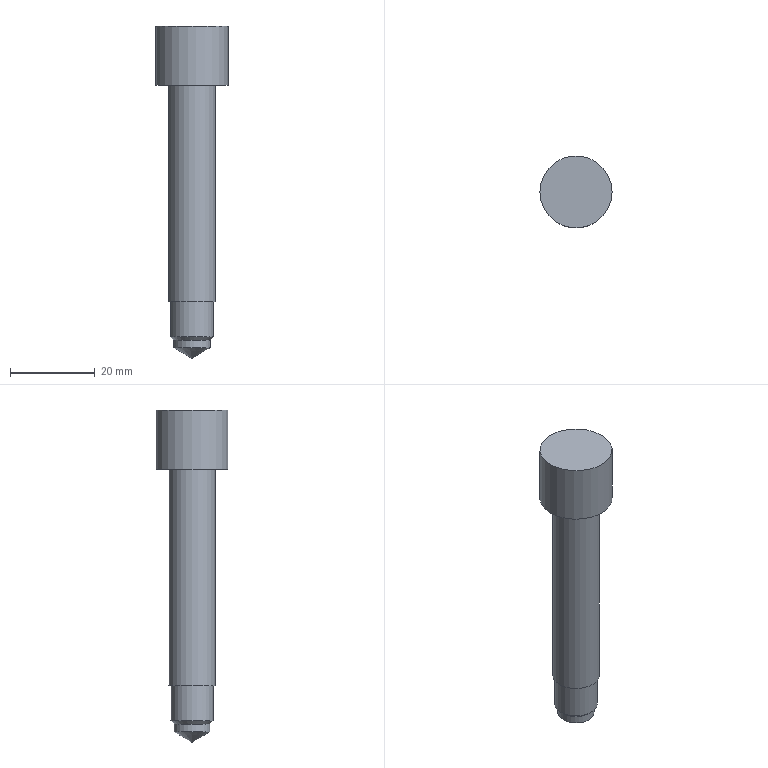Part | NX | features BREP 2 | 2 solids | 21 faces | box 17 x 17 x 78.231 mm | volume 15034 mm3 | plane 14 | cylinder 5 | cone 2 | commonest cylinder face diameters 8.5 x1 10 x1 11 x1 16 x1 17 x1
STEP:
#1=CARTESIAN_POINT('',(-4.25,0.,0.));
#2=VERTEX_POINT('',#1);
#3=CARTESIAN_POINT('',(0.,0.,0.));
#4=DIRECTION('',(0.,0.,1.));
#5=DIRECTION('',(-1.,0.,0.));
#6=AXIS2_PLACEMENT_3D('',#3,#4,#5);
#7=CIRCLE('',#6,4.25);
#8=EDGE_CURVE('',#2,#2,#7,.T.);
#9=ORIENTED_EDGE('',*,*,#8,.F.);
#10=EDGE_LOOP('',(#9));
#11=FACE_BOUND('',#10,.T.);
#12=CARTESIAN_POINT('',(-4.25,0.,-10.8));
#13=VERTEX_POINT('',#12);
#14=CARTESIAN_POINT('',(0.,0.,-10.8));
#15=DIRECTION('',(0.,0.,-1.));
#16=DIRECTION('',(-1.,0.,0.));
#17=AXIS2_PLACEMENT_3D('',#14,#15,#16);
#18=CIRCLE('',#17,4.25);
#19=EDGE_CURVE('',#13,#13,#18,.T.);
#20=ORIENTED_EDGE('',*,*,#19,.F.);
#21=EDGE_LOOP('',(#20));
#22=FACE_BOUND('',#21,.T.);
#23=CARTESIAN_POINT('',(0.,0.,-10.8));
#24=DIRECTION('',(0.,0.,1.));
#25=DIRECTION('',(-1.,0.,0.));
#26=AXIS2_PLACEMENT_3D('',#23,#24,#25);
#27=CYLINDRICAL_SURFACE('',#26,4.25);
#28=ADVANCED_FACE('',(#11,#22),#27,.T.);
#29=CARTESIAN_POINT('',(-0.2034,0.,-13.231));
#30=VERTEX_POINT('',#29);
#31=CARTESIAN_POINT('',(0.,0.,-13.231));
#32=DIRECTION('',(0.,0.,-1.));
#33=DIRECTION('',(-1.,0.,0.));
#34=AXIS2_PLACEMENT_3D('',#31,#32,#33);
#35=CIRCLE('',#34,0.2034);
#36=EDGE_CURVE('',#30,#30,#35,.T.);
#37=ORIENTED_EDGE('',*,*,#36,.T.);
#38=EDGE_LOOP('',(#37));
#39=FACE_BOUND('',#38,.T.);
#40=CARTESIAN_POINT('',(0.,0.,-13.231));
#41=DIRECTION('',(0.,0.,-1.));
#42=DIRECTION('',(1.,0.,0.));
#43=AXIS2_PLACEMENT_3D('',#40,#41,#42);
#44=PLANE('',#43);
#45=ADVANCED_FACE('',(#39),#44,.T.);
#46=ORIENTED_EDGE('',*,*,#36,.F.);
#47=EDGE_LOOP('',(#46));
#48=FACE_BOUND('',#47,.T.);
#49=ORIENTED_EDGE('',*,*,#19,.T.);
#50=EDGE_LOOP('',(#49));
#51=FACE_BOUND('',#50,.T.);
#52=CARTESIAN_POINT('',(0.,0.,-10.8));
#53=DIRECTION('',(0.,0.,1.));
#54=DIRECTION('',(-1.,0.,0.));
#55=AXIS2_PLACEMENT_3D('',#52,#53,#54);
#56=CONICAL_SURFACE('',#55,4.25,1.03);
#57=ADVANCED_FACE('',(#48,#51),#56,.T.);
#58=ORIENTED_EDGE('',*,*,#8,.T.);
#59=EDGE_LOOP('',(#58));
#60=FACE_BOUND('',#59,.T.);
#61=CARTESIAN_POINT('',(-5.5,0.,0.));
#62=VERTEX_POINT('',#61);
#63=CARTESIAN_POINT('',(0.,0.,0.));
#64=DIRECTION('',(0.,0.,-1.));
#65=DIRECTION('',(-1.,0.,0.));
#66=AXIS2_PLACEMENT_3D('',#63,#64,#65);
#67=CIRCLE('',#66,5.5);
#68=EDGE_CURVE('',#62,#62,#67,.T.);
#69=ORIENTED_EDGE('',*,*,#68,.T.);
#70=EDGE_LOOP('',(#69));
#71=FACE_BOUND('',#70,.T.);
#72=CARTESIAN_POINT('',(0.,0.,0.));
#73=DIRECTION('',(0.,0.,-1.));
#74=DIRECTION('',(1.,0.,0.));
#75=AXIS2_PLACEMENT_3D('',#72,#73,#74);
#76=PLANE('',#75);
#77=ADVANCED_FACE('',(#60,#71),#76,.T.);
#78=ORIENTED_EDGE('',*,*,#68,.F.);
#79=EDGE_LOOP('',(#78));
#80=FACE_BOUND('',#79,.T.);
#81=CARTESIAN_POINT('',(-5.5,0.,51.));
#82=VERTEX_POINT('',#81);
#83=CARTESIAN_POINT('',(0.,0.,51.));
#84=DIRECTION('',(0.,0.,-1.));
#85=DIRECTION('',(-1.,0.,0.));
#86=AXIS2_PLACEMENT_3D('',#83,#84,#85);
#87=CIRCLE('',#86,5.5);
#88=EDGE_CURVE('',#82,#82,#87,.T.);
#89=ORIENTED_EDGE('',*,*,#88,.T.);
#90=EDGE_LOOP('',(#89));
#91=FACE_BOUND('',#90,.T.);
#92=CARTESIAN_POINT('',(0.,0.,51.));
#93=DIRECTION('',(0.,0.,-1.));
#94=DIRECTION('',(1.,0.,0.));
#95=AXIS2_PLACEMENT_3D('',#92,#93,#94);
#96=CYLINDRICAL_SURFACE('',#95,5.5);
#97=ADVANCED_FACE('',(#80,#91),#96,.T.);
#98=CARTESIAN_POINT('',(8.5,0.,65.));
#99=VERTEX_POINT('',#98);
#100=CARTESIAN_POINT('',(0.,0.,65.));
#101=DIRECTION('',(0.,0.,1.));
#102=DIRECTION('',(1.,0.,0.));
#103=AXIS2_PLACEMENT_3D('',#100,#101,#102);
#104=CIRCLE('',#103,8.5);
#105=EDGE_CURVE('',#99,#99,#104,.T.);
#106=ORIENTED_EDGE('',*,*,#105,.T.);
#107=EDGE_LOOP('',(#106));
#108=FACE_BOUND('',#107,.T.);
#109=CARTESIAN_POINT('',(0.,0.,65.));
#110=DIRECTION('',(0.,0.,1.));
#111=DIRECTION('',(-1.,0.,0.));
#112=AXIS2_PLACEMENT_3D('',#109,#110,#111);
#113=PLANE('',#112);
#114=ADVANCED_FACE('',(#108),#113,.T.);
#115=ORIENTED_EDGE('',*,*,#105,.F.);
#116=EDGE_LOOP('',(#115));
#117=FACE_BOUND('',#116,.T.);
#118=CARTESIAN_POINT('',(8.5,0.,51.));
#119=VERTEX_POINT('',#118);
#120=CARTESIAN_POINT('',(0.,0.,51.));
#121=DIRECTION('',(0.,0.,1.));
#122=DIRECTION('',(1.,0.,0.));
#123=AXIS2_PLACEMENT_3D('',#120,#121,#122);
#124=CIRCLE('',#123,8.5);
#125=EDGE_CURVE('',#119,#119,#124,.T.);
#126=ORIENTED_EDGE('',*,*,#125,.T.);
#127=EDGE_LOOP('',(#126));
#128=FACE_BOUND('',#127,.T.);
#129=CARTESIAN_POINT('',(0.,0.,51.));
#130=DIRECTION('',(0.,0.,1.));
#131=DIRECTION('',(-1.,0.,0.));
#132=AXIS2_PLACEMENT_3D('',#129,#130,#131);
#133=CYLINDRICAL_SURFACE('',#132,8.5);
#134=ADVANCED_FACE('',(#117,#128),#133,.T.);
#135=ORIENTED_EDGE('',*,*,#88,.F.);
#136=EDGE_LOOP('',(#135));
#137=FACE_BOUND('',#136,.T.);
#138=ORIENTED_EDGE('',*,*,#125,.F.);
#139=EDGE_LOOP('',(#138));
#140=FACE_BOUND('',#139,.T.);
#141=CARTESIAN_POINT('',(0.,0.,51.));
#142=DIRECTION('',(0.,0.,-1.));
#143=DIRECTION('',(1.,0.,0.));
#144=AXIS2_PLACEMENT_3D('',#141,#142,#143);
#145=PLANE('',#144);
#146=ADVANCED_FACE('',(#137,#140),#145,.T.);
#147=CLOSED_SHELL('',(#28,#45,#57,#77,#97,#114,#134,#146));
#148=MANIFOLD_SOLID_BREP('',#147);
#149=CARTESIAN_POINT('',(8.,0.,61.));
#150=VERTEX_POINT('',#149);
#151=CARTESIAN_POINT('',(0.,0.,61.));
#152=DIRECTION('',(0.,0.,1.));
#153=DIRECTION('',(1.,0.,0.));
#154=AXIS2_PLACEMENT_3D('',#151,#152,#153);
#155=CIRCLE('',#154,8.);
#156=EDGE_CURVE('',#150,#150,#155,.T.);
#157=ORIENTED_EDGE('',*,*,#156,.T.);
#158=EDGE_LOOP('',(#157));
#159=FACE_BOUND('',#158,.T.);
#160=CARTESIAN_POINT('',(4.619,0.,61.));
#161=VERTEX_POINT('',#160);
#162=CARTESIAN_POINT('',(2.309,-4.,61.));
#163=VERTEX_POINT('',#162);
#164=CARTESIAN_POINT('',(4.619,0.,61.));
#165=DIRECTION('',(-0.5,-0.866,0.));
#166=VECTOR('',#165,1000.);
#167=LINE('',#164,#166);
#168=EDGE_CURVE('',#161,#163,#167,.T.);
#169=ORIENTED_EDGE('',*,*,#168,.T.);
#170=CARTESIAN_POINT('',(-2.309,-4.,61.));
#171=VERTEX_POINT('',#170);
#172=CARTESIAN_POINT('',(2.309,-4.,61.));
#173=DIRECTION('',(-1.,0.,0.));
#174=VECTOR('',#173,1000.);
#175=LINE('',#172,#174);
#176=EDGE_CURVE('',#163,#171,#175,.T.);
#177=ORIENTED_EDGE('',*,*,#176,.T.);
#178=CARTESIAN_POINT('',(-4.619,0.,61.));
#179=VERTEX_POINT('',#178);
#180=CARTESIAN_POINT('',(-2.309,-4.,61.));
#181=DIRECTION('',(-0.5,0.866,0.));
#182=VECTOR('',#181,1000.);
#183=LINE('',#180,#182);
#184=EDGE_CURVE('',#171,#179,#183,.T.);
#185=ORIENTED_EDGE('',*,*,#184,.T.);
#186=CARTESIAN_POINT('',(-2.309,4.,61.));
#187=VERTEX_POINT('',#186);
#188=CARTESIAN_POINT('',(-4.619,0.,61.));
#189=DIRECTION('',(0.5,0.866,0.));
#190=VECTOR('',#189,1000.);
#191=LINE('',#188,#190);
#192=EDGE_CURVE('',#179,#187,#191,.T.);
#193=ORIENTED_EDGE('',*,*,#192,.T.);
#194=CARTESIAN_POINT('',(2.309,4.,61.));
#195=VERTEX_POINT('',#194);
#196=CARTESIAN_POINT('',(-2.309,4.,61.));
#197=DIRECTION('',(1.,0.,0.));
#198=VECTOR('',#197,1000.);
#199=LINE('',#196,#198);
#200=EDGE_CURVE('',#187,#195,#199,.T.);
#201=ORIENTED_EDGE('',*,*,#200,.T.);
#202=CARTESIAN_POINT('',(2.309,4.,61.));
#203=DIRECTION('',(0.5,-0.866,0.));
#204=VECTOR('',#203,1000.);
#205=LINE('',#202,#204);
#206=EDGE_CURVE('',#195,#161,#205,.T.);
#207=ORIENTED_EDGE('',*,*,#206,.T.);
#208=EDGE_LOOP('',(#169,#177,#185,#193,#201,#207));
#209=FACE_BOUND('',#208,.T.);
#210=CARTESIAN_POINT('',(0.,0.,61.));
#211=DIRECTION('',(0.,0.,1.));
#212=DIRECTION('',(-1.,0.,0.));
#213=AXIS2_PLACEMENT_3D('',#210,#211,#212);
#214=PLANE('',#213);
#215=ADVANCED_FACE('',(#159,#209),#214,.T.);
#216=CARTESIAN_POINT('',(5.,0.,-8.25));
#217=VERTEX_POINT('',#216);
#218=CARTESIAN_POINT('',(0.,0.,-8.25));
#219=DIRECTION('',(0.,0.,1.));
#220=DIRECTION('',(1.,0.,0.));
#221=AXIS2_PLACEMENT_3D('',#218,#219,#220);
#222=CIRCLE('',#221,5.);
#223=EDGE_CURVE('',#217,#217,#222,.T.);
#224=ORIENTED_EDGE('',*,*,#223,.T.);
#225=EDGE_LOOP('',(#224));
#226=FACE_BOUND('',#225,.T.);
#227=CARTESIAN_POINT('',(5.,0.,51.));
#228=VERTEX_POINT('',#227);
#229=CARTESIAN_POINT('',(0.,0.,51.));
#230=DIRECTION('',(0.,0.,1.));
#231=DIRECTION('',(1.,0.,0.));
#232=AXIS2_PLACEMENT_3D('',#229,#230,#231);
#233=CIRCLE('',#232,5.);
#234=EDGE_CURVE('',#228,#228,#233,.T.);
#235=ORIENTED_EDGE('',*,*,#234,.F.);
#236=EDGE_LOOP('',(#235));
#237=FACE_BOUND('',#236,.T.);
#238=CARTESIAN_POINT('',(0.,0.,-9.));
#239=DIRECTION('',(0.,0.,1.));
#240=DIRECTION('',(-1.,0.,0.));
#241=AXIS2_PLACEMENT_3D('',#238,#239,#240);
#242=CYLINDRICAL_SURFACE('',#241,5.);
#243=ADVANCED_FACE('',(#226,#237),#242,.T.);
#244=CARTESIAN_POINT('',(4.25,0.,-9.));
#245=VERTEX_POINT('',#244);
#246=CARTESIAN_POINT('',(0.,0.,-9.));
#247=DIRECTION('',(0.,0.,-1.));
#248=DIRECTION('',(1.,0.,0.));
#249=AXIS2_PLACEMENT_3D('',#246,#247,#248);
#250=CIRCLE('',#249,4.25);
#251=EDGE_CURVE('',#245,#245,#250,.T.);
#252=ORIENTED_EDGE('',*,*,#251,.T.);
#253=EDGE_LOOP('',(#252));
#254=FACE_BOUND('',#253,.T.);
#255=CARTESIAN_POINT('',(0.,0.,-9.));
#256=DIRECTION('',(0.,0.,1.));
#257=DIRECTION('',(-1.,0.,0.));
#258=AXIS2_PLACEMENT_3D('',#255,#256,#257);
#259=PLANE('',#258);
#260=ADVANCED_FACE('',(#254),#259,.F.);
#261=ORIENTED_EDGE('',*,*,#234,.T.);
#262=EDGE_LOOP('',(#261));
#263=FACE_BOUND('',#262,.T.);
#264=CARTESIAN_POINT('',(8.,0.,51.));
#265=VERTEX_POINT('',#264);
#266=CARTESIAN_POINT('',(0.,0.,51.));
#267=DIRECTION('',(0.,0.,1.));
#268=DIRECTION('',(1.,0.,0.));
#269=AXIS2_PLACEMENT_3D('',#266,#267,#268);
#270=CIRCLE('',#269,8.);
#271=EDGE_CURVE('',#265,#265,#270,.T.);
#272=ORIENTED_EDGE('',*,*,#271,.F.);
#273=EDGE_LOOP('',(#272));
#274=FACE_BOUND('',#273,.T.);
#275=CARTESIAN_POINT('',(0.,0.,51.));
#276=DIRECTION('',(0.,0.,-1.));
#277=DIRECTION('',(1.,0.,0.));
#278=AXIS2_PLACEMENT_3D('',#275,#276,#277);
#279=PLANE('',#278);
#280=ADVANCED_FACE('',(#263,#274),#279,.T.);
#281=ORIENTED_EDGE('',*,*,#156,.F.);
#282=EDGE_LOOP('',(#281));
#283=FACE_BOUND('',#282,.T.);
#284=ORIENTED_EDGE('',*,*,#271,.T.);
#285=EDGE_LOOP('',(#284));
#286=FACE_BOUND('',#285,.T.);
#287=CARTESIAN_POINT('',(0.,0.,51.));
#288=DIRECTION('',(0.,0.,1.));
#289=DIRECTION('',(-1.,0.,0.));
#290=AXIS2_PLACEMENT_3D('',#287,#288,#289);
#291=CYLINDRICAL_SURFACE('',#290,8.);
#292=ADVANCED_FACE('',(#283,#286),#291,.T.);
#293=ORIENTED_EDGE('',*,*,#251,.F.);
#294=EDGE_LOOP('',(#293));
#295=FACE_BOUND('',#294,.T.);
#296=ORIENTED_EDGE('',*,*,#223,.F.);
#297=EDGE_LOOP('',(#296));
#298=FACE_BOUND('',#297,.T.);
#299=CARTESIAN_POINT('',(0.,0.,-8.25));
#300=DIRECTION('',(0.,0.,1.));
#301=DIRECTION('',(-1.,0.,0.));
#302=AXIS2_PLACEMENT_3D('',#299,#300,#301);
#303=CONICAL_SURFACE('',#302,5.,0.7854);
#304=ADVANCED_FACE('',(#295,#298),#303,.T.);
#305=ORIENTED_EDGE('',*,*,#176,.F.);
#306=CARTESIAN_POINT('',(2.309,-4.,54.4));
#307=VERTEX_POINT('',#306);
#308=CARTESIAN_POINT('',(2.309,-4.,54.4));
#309=DIRECTION('',(0.,0.,1.));
#310=VECTOR('',#309,1000.);
#311=LINE('',#308,#310);
#312=EDGE_CURVE('',#307,#163,#311,.T.);
#313=ORIENTED_EDGE('',*,*,#312,.F.);
#314=CARTESIAN_POINT('',(-2.309,-4.,54.4));
#315=VERTEX_POINT('',#314);
#316=CARTESIAN_POINT('',(2.309,-4.,54.4));
#317=DIRECTION('',(-1.,0.,0.));
#318=VECTOR('',#317,1000.);
#319=LINE('',#316,#318);
#320=EDGE_CURVE('',#307,#315,#319,.T.);
#321=ORIENTED_EDGE('',*,*,#320,.T.);
#322=CARTESIAN_POINT('',(-2.309,-4.,54.4));
#323=DIRECTION('',(0.,0.,1.));
#324=VECTOR('',#323,1000.);
#325=LINE('',#322,#324);
#326=EDGE_CURVE('',#315,#171,#325,.T.);
#327=ORIENTED_EDGE('',*,*,#326,.T.);
#328=EDGE_LOOP('',(#305,#313,#321,#327));
#329=FACE_BOUND('',#328,.T.);
#330=CARTESIAN_POINT('',(2.309,-4.,54.4));
#331=DIRECTION('',(0.,1.,0.));
#332=DIRECTION('',(0.,0.,-1.));
#333=AXIS2_PLACEMENT_3D('',#330,#331,#332);
#334=PLANE('',#333);
#335=ADVANCED_FACE('',(#329),#334,.T.);
#336=ORIENTED_EDGE('',*,*,#184,.F.);
#337=ORIENTED_EDGE('',*,*,#326,.F.);
#338=CARTESIAN_POINT('',(-4.619,0.,54.4));
#339=VERTEX_POINT('',#338);
#340=CARTESIAN_POINT('',(-2.309,-4.,54.4));
#341=DIRECTION('',(-0.5,0.866,0.));
#342=VECTOR('',#341,1000.);
#343=LINE('',#340,#342);
#344=EDGE_CURVE('',#315,#339,#343,.T.);
#345=ORIENTED_EDGE('',*,*,#344,.T.);
#346=CARTESIAN_POINT('',(-4.619,0.,54.4));
#347=DIRECTION('',(0.,0.,1.));
#348=VECTOR('',#347,1000.);
#349=LINE('',#346,#348);
#350=EDGE_CURVE('',#339,#179,#349,.T.);
#351=ORIENTED_EDGE('',*,*,#350,.T.);
#352=EDGE_LOOP('',(#336,#337,#345,#351));
#353=FACE_BOUND('',#352,.T.);
#354=CARTESIAN_POINT('',(-2.309,-4.,54.4));
#355=DIRECTION('',(0.866,0.5,0.));
#356=DIRECTION('',(0.5,-0.866,0.));
#357=AXIS2_PLACEMENT_3D('',#354,#355,#356);
#358=PLANE('',#357);
#359=ADVANCED_FACE('',(#353),#358,.T.);
#360=ORIENTED_EDGE('',*,*,#192,.F.);
#361=ORIENTED_EDGE('',*,*,#350,.F.);
#362=CARTESIAN_POINT('',(-2.309,4.,54.4));
#363=VERTEX_POINT('',#362);
#364=CARTESIAN_POINT('',(-4.619,0.,54.4));
#365=DIRECTION('',(0.5,0.866,0.));
#366=VECTOR('',#365,1000.);
#367=LINE('',#364,#366);
#368=EDGE_CURVE('',#339,#363,#367,.T.);
#369=ORIENTED_EDGE('',*,*,#368,.T.);
#370=CARTESIAN_POINT('',(-2.309,4.,54.4));
#371=DIRECTION('',(0.,0.,1.));
#372=VECTOR('',#371,1000.);
#373=LINE('',#370,#372);
#374=EDGE_CURVE('',#363,#187,#373,.T.);
#375=ORIENTED_EDGE('',*,*,#374,.T.);
#376=EDGE_LOOP('',(#360,#361,#369,#375));
#377=FACE_BOUND('',#376,.T.);
#378=CARTESIAN_POINT('',(-4.619,0.,54.4));
#379=DIRECTION('',(0.866,-0.5,0.));
#380=DIRECTION('',(-0.5,-0.866,0.));
#381=AXIS2_PLACEMENT_3D('',#378,#379,#380);
#382=PLANE('',#381);
#383=ADVANCED_FACE('',(#377),#382,.T.);
#384=ORIENTED_EDGE('',*,*,#200,.F.);
#385=ORIENTED_EDGE('',*,*,#374,.F.);
#386=CARTESIAN_POINT('',(2.309,4.,54.4));
#387=VERTEX_POINT('',#386);
#388=CARTESIAN_POINT('',(-2.309,4.,54.4));
#389=DIRECTION('',(1.,0.,0.));
#390=VECTOR('',#389,1000.);
#391=LINE('',#388,#390);
#392=EDGE_CURVE('',#363,#387,#391,.T.);
#393=ORIENTED_EDGE('',*,*,#392,.T.);
#394=CARTESIAN_POINT('',(2.309,4.,54.4));
#395=DIRECTION('',(0.,0.,1.));
#396=VECTOR('',#395,1000.);
#397=LINE('',#394,#396);
#398=EDGE_CURVE('',#387,#195,#397,.T.);
#399=ORIENTED_EDGE('',*,*,#398,.T.);
#400=EDGE_LOOP('',(#384,#385,#393,#399));
#401=FACE_BOUND('',#400,.T.);
#402=CARTESIAN_POINT('',(-2.309,4.,54.4));
#403=DIRECTION('',(0.,-1.,0.));
#404=DIRECTION('',(0.,0.,1.));
#405=AXIS2_PLACEMENT_3D('',#402,#403,#404);
#406=PLANE('',#405);
#407=ADVANCED_FACE('',(#401),#406,.T.);
#408=ORIENTED_EDGE('',*,*,#206,.F.);
#409=ORIENTED_EDGE('',*,*,#398,.F.);
#410=CARTESIAN_POINT('',(4.619,0.,54.4));
#411=VERTEX_POINT('',#410);
#412=CARTESIAN_POINT('',(2.309,4.,54.4));
#413=DIRECTION('',(0.5,-0.866,0.));
#414=VECTOR('',#413,1000.);
#415=LINE('',#412,#414);
#416=EDGE_CURVE('',#387,#411,#415,.T.);
#417=ORIENTED_EDGE('',*,*,#416,.T.);
#418=CARTESIAN_POINT('',(4.619,0.,54.4));
#419=DIRECTION('',(0.,0.,1.));
#420=VECTOR('',#419,1000.);
#421=LINE('',#418,#420);
#422=EDGE_CURVE('',#411,#161,#421,.T.);
#423=ORIENTED_EDGE('',*,*,#422,.T.);
#424=EDGE_LOOP('',(#408,#409,#417,#423));
#425=FACE_BOUND('',#424,.T.);
#426=CARTESIAN_POINT('',(2.309,4.,54.4));
#427=DIRECTION('',(-0.866,-0.5,0.));
#428=DIRECTION('',(-0.5,0.866,0.));
#429=AXIS2_PLACEMENT_3D('',#426,#427,#428);
#430=PLANE('',#429);
#431=ADVANCED_FACE('',(#425),#430,.T.);
#432=ORIENTED_EDGE('',*,*,#168,.F.);
#433=ORIENTED_EDGE('',*,*,#422,.F.);
#434=CARTESIAN_POINT('',(4.619,0.,54.4));
#435=DIRECTION('',(-0.5,-0.866,0.));
#436=VECTOR('',#435,1000.);
#437=LINE('',#434,#436);
#438=EDGE_CURVE('',#411,#307,#437,.T.);
#439=ORIENTED_EDGE('',*,*,#438,.T.);
#440=ORIENTED_EDGE('',*,*,#312,.T.);
#441=EDGE_LOOP('',(#432,#433,#439,#440));
#442=FACE_BOUND('',#441,.T.);
#443=CARTESIAN_POINT('',(4.619,0.,54.4));
#444=DIRECTION('',(-0.866,0.5,0.));
#445=DIRECTION('',(0.5,0.866,0.));
#446=AXIS2_PLACEMENT_3D('',#443,#444,#445);
#447=PLANE('',#446);
#448=ADVANCED_FACE('',(#442),#447,.T.);
#449=ORIENTED_EDGE('',*,*,#320,.F.);
#450=ORIENTED_EDGE('',*,*,#438,.F.);
#451=ORIENTED_EDGE('',*,*,#416,.F.);
#452=ORIENTED_EDGE('',*,*,#392,.F.);
#453=ORIENTED_EDGE('',*,*,#368,.F.);
#454=ORIENTED_EDGE('',*,*,#344,.F.);
#455=EDGE_LOOP('',(#449,#450,#451,#452,#453,#454));
#456=FACE_BOUND('',#455,.T.);
#457=CARTESIAN_POINT('',(-6.928,-4.,54.4));
#458=DIRECTION('',(0.,0.,-1.));
#459=DIRECTION('',(1.,0.,0.));
#460=AXIS2_PLACEMENT_3D('',#457,#458,#459);
#461=PLANE('',#460);
#462=ADVANCED_FACE('',(#456),#461,.F.);
#463=CLOSED_SHELL('',(#215,#243,#260,#280,#292,#304,#335,#359,#383,#407,#431,#448,#462));
#464=MANIFOLD_SOLID_BREP('',#463);
#465=(LENGTH_UNIT()NAMED_UNIT(*)SI_UNIT(.MILLI.,.METRE.));
#466=UNCERTAINTY_MEASURE_WITH_UNIT(LENGTH_MEASURE(0.00001),#465,'','');
#467=(NAMED_UNIT(*)PLANE_ANGLE_UNIT()SI_UNIT($,.RADIAN.));
#468=(NAMED_UNIT(*)SI_UNIT($,.STERADIAN.)SOLID_ANGLE_UNIT());
#469=(GEOMETRIC_REPRESENTATION_CONTEXT(3)GLOBAL_UNCERTAINTY_ASSIGNED_CONTEXT((#466))GLOBAL_UNIT_ASSIGNED_CONTEXT((#465,#467,#468))REPRESENTATION_CONTEXT('',''));
#470=ADVANCED_BREP_SHAPE_REPRESENTATION('',(#148,#464),#469);